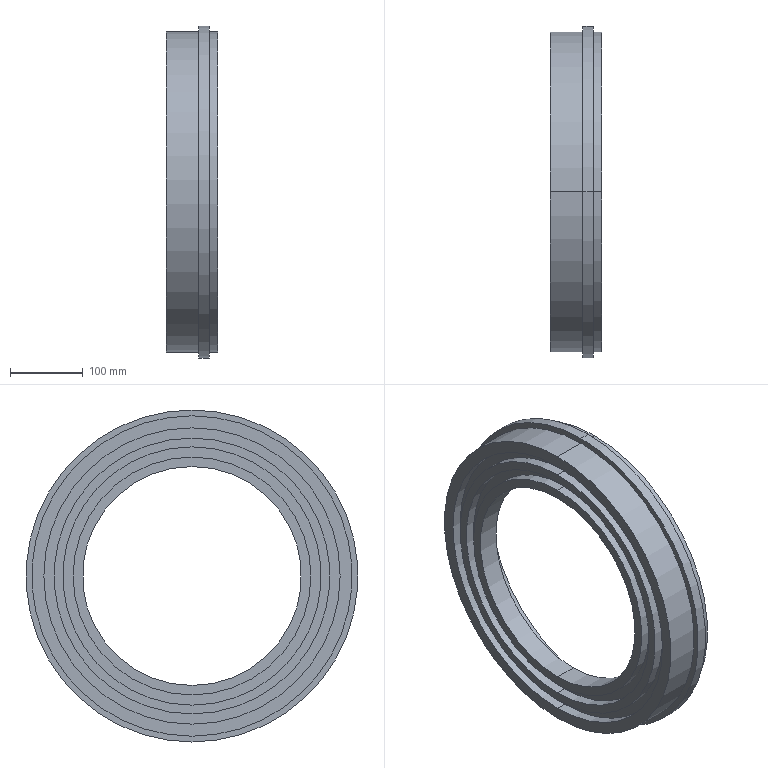Part | SolidWorks | features Revolution 1 | 1 solid | 27 faces | box 71 x 455 x 455 mm | volume 3180516 mm3 | cylinder 18 | plane 9 | commonest cylinder face diameters 439 x4 300 x2 326 x2 354 x2 378 x2 400 x2
STEP:
#1=CARTESIAN_POINT('',(71.,0.,-200.));
#2=VERTEX_POINT('',#1);
#3=CARTESIAN_POINT('',(71.,0.,200.));
#4=VERTEX_POINT('',#3);
#5=CARTESIAN_POINT('',(71.,0.,0.));
#6=DIRECTION('',(-1.,0.,0.));
#7=DIRECTION('',(0.,0.,1.));
#8=AXIS2_PLACEMENT_3D('',#5,#6,#7);
#9=CIRCLE('',#8,200.);
#10=EDGE_CURVE('',#2,#4,#9,.T.);
#11=ORIENTED_EDGE('',*,*,#10,.F.);
#12=CARTESIAN_POINT('',(30.,0.,-200.));
#13=VERTEX_POINT('',#12);
#14=CARTESIAN_POINT('',(0.,0.,-200.));
#15=DIRECTION('',(-1.,0.,0.));
#16=VECTOR('',#15,1000.);
#17=LINE('',#14,#16);
#18=EDGE_CURVE('',#2,#13,#17,.T.);
#19=ORIENTED_EDGE('',*,*,#18,.T.);
#20=CARTESIAN_POINT('',(30.,0.,200.));
#21=VERTEX_POINT('',#20);
#22=CARTESIAN_POINT('',(30.,0.,0.));
#23=DIRECTION('',(-1.,0.,0.));
#24=DIRECTION('',(0.,0.,1.));
#25=AXIS2_PLACEMENT_3D('',#22,#23,#24);
#26=CIRCLE('',#25,200.);
#27=EDGE_CURVE('',#13,#21,#26,.T.);
#28=ORIENTED_EDGE('',*,*,#27,.T.);
#29=CARTESIAN_POINT('',(0.,0.,200.));
#30=DIRECTION('',(-1.,0.,0.));
#31=VECTOR('',#30,1000.);
#32=LINE('',#29,#31);
#33=EDGE_CURVE('',#4,#21,#32,.T.);
#34=ORIENTED_EDGE('',*,*,#33,.F.);
#35=EDGE_LOOP('',(#11,#19,#28,#34));
#36=FACE_OUTER_BOUND('',#35,.T.);
#37=CARTESIAN_POINT('',(0.,0.,0.));
#38=DIRECTION('',(-1.,0.,0.));
#39=DIRECTION('',(0.,0.,1.));
#40=AXIS2_PLACEMENT_3D('',#37,#38,#39);
#41=CYLINDRICAL_SURFACE('',#40,200.);
#42=ADVANCED_FACE('',(#36),#41,.F.);
#43=CARTESIAN_POINT('',(71.,0.,219.5));
#44=VERTEX_POINT('',#43);
#45=CARTESIAN_POINT('',(71.,0.,-219.5));
#46=VERTEX_POINT('',#45);
#47=CARTESIAN_POINT('',(71.,0.,0.));
#48=DIRECTION('',(-1.,0.,0.));
#49=DIRECTION('',(0.,0.,1.));
#50=AXIS2_PLACEMENT_3D('',#47,#48,#49);
#51=CIRCLE('',#50,219.5);
#52=EDGE_CURVE('',#44,#46,#51,.T.);
#53=ORIENTED_EDGE('',*,*,#52,.T.);
#54=CARTESIAN_POINT('',(59.,0.,-219.5));
#55=VERTEX_POINT('',#54);
#56=CARTESIAN_POINT('',(0.,0.,-219.5));
#57=DIRECTION('',(-1.,0.,0.));
#58=VECTOR('',#57,1000.);
#59=LINE('',#56,#58);
#60=EDGE_CURVE('',#46,#55,#59,.T.);
#61=ORIENTED_EDGE('',*,*,#60,.T.);
#62=CARTESIAN_POINT('',(59.,0.,219.5));
#63=VERTEX_POINT('',#62);
#64=CARTESIAN_POINT('',(59.,0.,0.));
#65=DIRECTION('',(-1.,0.,0.));
#66=DIRECTION('',(0.,0.,1.));
#67=AXIS2_PLACEMENT_3D('',#64,#65,#66);
#68=CIRCLE('',#67,219.5);
#69=EDGE_CURVE('',#63,#55,#68,.T.);
#70=ORIENTED_EDGE('',*,*,#69,.F.);
#71=CARTESIAN_POINT('',(0.,0.,219.5));
#72=DIRECTION('',(-1.,0.,0.));
#73=VECTOR('',#72,1000.);
#74=LINE('',#71,#73);
#75=EDGE_CURVE('',#44,#63,#74,.T.);
#76=ORIENTED_EDGE('',*,*,#75,.F.);
#77=EDGE_LOOP('',(#53,#61,#70,#76));
#78=FACE_OUTER_BOUND('',#77,.T.);
#79=CARTESIAN_POINT('',(0.,0.,0.));
#80=DIRECTION('',(-1.,0.,0.));
#81=DIRECTION('',(0.,0.,1.));
#82=AXIS2_PLACEMENT_3D('',#79,#80,#81);
#83=CYLINDRICAL_SURFACE('',#82,219.5);
#84=ADVANCED_FACE('',(#78),#83,.T.);
#85=CARTESIAN_POINT('',(59.,0.,227.5));
#86=VERTEX_POINT('',#85);
#87=CARTESIAN_POINT('',(59.,0.,-227.5));
#88=VERTEX_POINT('',#87);
#89=CARTESIAN_POINT('',(59.,0.,0.));
#90=DIRECTION('',(-1.,0.,0.));
#91=DIRECTION('',(0.,0.,1.));
#92=AXIS2_PLACEMENT_3D('',#89,#90,#91);
#93=CIRCLE('',#92,227.5);
#94=EDGE_CURVE('',#86,#88,#93,.T.);
#95=ORIENTED_EDGE('',*,*,#94,.T.);
#96=CARTESIAN_POINT('',(45.,0.,-227.5));
#97=VERTEX_POINT('',#96);
#98=CARTESIAN_POINT('',(0.,0.,-227.5));
#99=DIRECTION('',(-1.,0.,0.));
#100=VECTOR('',#99,1000.);
#101=LINE('',#98,#100);
#102=EDGE_CURVE('',#88,#97,#101,.T.);
#103=ORIENTED_EDGE('',*,*,#102,.T.);
#104=CARTESIAN_POINT('',(45.,0.,227.5));
#105=VERTEX_POINT('',#104);
#106=CARTESIAN_POINT('',(45.,0.,0.));
#107=DIRECTION('',(-1.,0.,0.));
#108=DIRECTION('',(0.,0.,1.));
#109=AXIS2_PLACEMENT_3D('',#106,#107,#108);
#110=CIRCLE('',#109,227.5);
#111=EDGE_CURVE('',#105,#97,#110,.T.);
#112=ORIENTED_EDGE('',*,*,#111,.F.);
#113=CARTESIAN_POINT('',(0.,0.,227.5));
#114=DIRECTION('',(-1.,0.,0.));
#115=VECTOR('',#114,1000.);
#116=LINE('',#113,#115);
#117=EDGE_CURVE('',#86,#105,#116,.T.);
#118=ORIENTED_EDGE('',*,*,#117,.F.);
#119=EDGE_LOOP('',(#95,#103,#112,#118));
#120=FACE_OUTER_BOUND('',#119,.T.);
#121=CARTESIAN_POINT('',(0.,0.,0.));
#122=DIRECTION('',(-1.,0.,0.));
#123=DIRECTION('',(0.,0.,1.));
#124=AXIS2_PLACEMENT_3D('',#121,#122,#123);
#125=CYLINDRICAL_SURFACE('',#124,227.5);
#126=ADVANCED_FACE('',(#120),#125,.T.);
#127=CARTESIAN_POINT('',(45.,0.,219.5));
#128=VERTEX_POINT('',#127);
#129=CARTESIAN_POINT('',(45.,0.,-219.5));
#130=VERTEX_POINT('',#129);
#131=CARTESIAN_POINT('',(45.,0.,0.));
#132=DIRECTION('',(-1.,0.,0.));
#133=DIRECTION('',(0.,0.,1.));
#134=AXIS2_PLACEMENT_3D('',#131,#132,#133);
#135=CIRCLE('',#134,219.5);
#136=EDGE_CURVE('',#128,#130,#135,.T.);
#137=ORIENTED_EDGE('',*,*,#136,.T.);
#138=CARTESIAN_POINT('',(0.,0.,-219.5));
#139=VERTEX_POINT('',#138);
#140=CARTESIAN_POINT('',(0.,0.,-219.5));
#141=DIRECTION('',(-1.,0.,0.));
#142=VECTOR('',#141,1000.);
#143=LINE('',#140,#142);
#144=EDGE_CURVE('',#130,#139,#143,.T.);
#145=ORIENTED_EDGE('',*,*,#144,.T.);
#146=CARTESIAN_POINT('',(0.,0.,219.5));
#147=VERTEX_POINT('',#146);
#148=CARTESIAN_POINT('',(0.,0.,0.));
#149=DIRECTION('',(-1.,0.,0.));
#150=DIRECTION('',(0.,0.,1.));
#151=AXIS2_PLACEMENT_3D('',#148,#149,#150);
#152=CIRCLE('',#151,219.5);
#153=EDGE_CURVE('',#147,#139,#152,.T.);
#154=ORIENTED_EDGE('',*,*,#153,.F.);
#155=CARTESIAN_POINT('',(0.,0.,219.5));
#156=DIRECTION('',(-1.,0.,0.));
#157=VECTOR('',#156,1000.);
#158=LINE('',#155,#157);
#159=EDGE_CURVE('',#128,#147,#158,.T.);
#160=ORIENTED_EDGE('',*,*,#159,.F.);
#161=EDGE_LOOP('',(#137,#145,#154,#160));
#162=FACE_OUTER_BOUND('',#161,.T.);
#163=CARTESIAN_POINT('',(0.,0.,0.));
#164=DIRECTION('',(-1.,0.,0.));
#165=DIRECTION('',(0.,0.,1.));
#166=AXIS2_PLACEMENT_3D('',#163,#164,#165);
#167=CYLINDRICAL_SURFACE('',#166,219.5);
#168=ADVANCED_FACE('',(#162),#167,.T.);
#169=CARTESIAN_POINT('',(14.,0.,-203.));
#170=VERTEX_POINT('',#169);
#171=CARTESIAN_POINT('',(14.,0.,203.));
#172=VERTEX_POINT('',#171);
#173=CARTESIAN_POINT('',(14.,0.,0.));
#174=DIRECTION('',(-1.,0.,0.));
#175=DIRECTION('',(0.,0.,1.));
#176=AXIS2_PLACEMENT_3D('',#173,#174,#175);
#177=CIRCLE('',#176,203.);
#178=EDGE_CURVE('',#170,#172,#177,.T.);
#179=ORIENTED_EDGE('',*,*,#178,.F.);
#180=CARTESIAN_POINT('',(0.,0.,-203.));
#181=VERTEX_POINT('',#180);
#182=CARTESIAN_POINT('',(0.,0.,-203.));
#183=DIRECTION('',(-1.,0.,0.));
#184=VECTOR('',#183,1000.);
#185=LINE('',#182,#184);
#186=EDGE_CURVE('',#170,#181,#185,.T.);
#187=ORIENTED_EDGE('',*,*,#186,.T.);
#188=CARTESIAN_POINT('',(0.,0.,203.));
#189=VERTEX_POINT('',#188);
#190=CARTESIAN_POINT('',(0.,0.,0.));
#191=DIRECTION('',(-1.,0.,0.));
#192=DIRECTION('',(0.,0.,1.));
#193=AXIS2_PLACEMENT_3D('',#190,#191,#192);
#194=CIRCLE('',#193,203.);
#195=EDGE_CURVE('',#181,#189,#194,.T.);
#196=ORIENTED_EDGE('',*,*,#195,.T.);
#197=CARTESIAN_POINT('',(0.,0.,203.));
#198=DIRECTION('',(-1.,0.,0.));
#199=VECTOR('',#198,1000.);
#200=LINE('',#197,#199);
#201=EDGE_CURVE('',#172,#189,#200,.T.);
#202=ORIENTED_EDGE('',*,*,#201,.F.);
#203=EDGE_LOOP('',(#179,#187,#196,#202));
#204=FACE_OUTER_BOUND('',#203,.T.);
#205=CARTESIAN_POINT('',(0.,0.,0.));
#206=DIRECTION('',(-1.,0.,0.));
#207=DIRECTION('',(0.,0.,1.));
#208=AXIS2_PLACEMENT_3D('',#205,#206,#207);
#209=CYLINDRICAL_SURFACE('',#208,203.);
#210=ADVANCED_FACE('',(#204),#209,.F.);
#211=CARTESIAN_POINT('',(14.,0.,189.));
#212=VERTEX_POINT('',#211);
#213=CARTESIAN_POINT('',(14.,0.,-189.));
#214=VERTEX_POINT('',#213);
#215=CARTESIAN_POINT('',(14.,0.,0.));
#216=DIRECTION('',(-1.,0.,0.));
#217=DIRECTION('',(0.,0.,1.));
#218=AXIS2_PLACEMENT_3D('',#215,#216,#217);
#219=CIRCLE('',#218,189.);
#220=EDGE_CURVE('',#212,#214,#219,.T.);
#221=ORIENTED_EDGE('',*,*,#220,.T.);
#222=CARTESIAN_POINT('',(0.,0.,-189.));
#223=VERTEX_POINT('',#222);
#224=CARTESIAN_POINT('',(0.,0.,-189.));
#225=DIRECTION('',(-1.,0.,0.));
#226=VECTOR('',#225,1000.);
#227=LINE('',#224,#226);
#228=EDGE_CURVE('',#214,#223,#227,.T.);
#229=ORIENTED_EDGE('',*,*,#228,.T.);
#230=CARTESIAN_POINT('',(0.,0.,189.));
#231=VERTEX_POINT('',#230);
#232=CARTESIAN_POINT('',(0.,0.,0.));
#233=DIRECTION('',(-1.,0.,0.));
#234=DIRECTION('',(0.,0.,1.));
#235=AXIS2_PLACEMENT_3D('',#232,#233,#234);
#236=CIRCLE('',#235,189.);
#237=EDGE_CURVE('',#231,#223,#236,.T.);
#238=ORIENTED_EDGE('',*,*,#237,.F.);
#239=CARTESIAN_POINT('',(0.,0.,189.));
#240=DIRECTION('',(-1.,0.,0.));
#241=VECTOR('',#240,1000.);
#242=LINE('',#239,#241);
#243=EDGE_CURVE('',#212,#231,#242,.T.);
#244=ORIENTED_EDGE('',*,*,#243,.F.);
#245=EDGE_LOOP('',(#221,#229,#238,#244));
#246=FACE_OUTER_BOUND('',#245,.T.);
#247=CARTESIAN_POINT('',(0.,0.,0.));
#248=DIRECTION('',(-1.,0.,0.));
#249=DIRECTION('',(0.,0.,1.));
#250=AXIS2_PLACEMENT_3D('',#247,#248,#249);
#251=CYLINDRICAL_SURFACE('',#250,189.);
#252=ADVANCED_FACE('',(#246),#251,.T.);
#253=CARTESIAN_POINT('',(14.,0.,-177.));
#254=VERTEX_POINT('',#253);
#255=CARTESIAN_POINT('',(14.,0.,177.));
#256=VERTEX_POINT('',#255);
#257=CARTESIAN_POINT('',(14.,0.,0.));
#258=DIRECTION('',(-1.,0.,0.));
#259=DIRECTION('',(0.,0.,1.));
#260=AXIS2_PLACEMENT_3D('',#257,#258,#259);
#261=CIRCLE('',#260,177.);
#262=EDGE_CURVE('',#254,#256,#261,.T.);
#263=ORIENTED_EDGE('',*,*,#262,.F.);
#264=CARTESIAN_POINT('',(0.,0.,-177.));
#265=VERTEX_POINT('',#264);
#266=CARTESIAN_POINT('',(0.,0.,-177.));
#267=DIRECTION('',(-1.,0.,0.));
#268=VECTOR('',#267,1000.);
#269=LINE('',#266,#268);
#270=EDGE_CURVE('',#254,#265,#269,.T.);
#271=ORIENTED_EDGE('',*,*,#270,.T.);
#272=CARTESIAN_POINT('',(0.,0.,177.));
#273=VERTEX_POINT('',#272);
#274=CARTESIAN_POINT('',(0.,0.,0.));
#275=DIRECTION('',(-1.,0.,0.));
#276=DIRECTION('',(0.,0.,1.));
#277=AXIS2_PLACEMENT_3D('',#274,#275,#276);
#278=CIRCLE('',#277,177.);
#279=EDGE_CURVE('',#265,#273,#278,.T.);
#280=ORIENTED_EDGE('',*,*,#279,.T.);
#281=CARTESIAN_POINT('',(0.,0.,177.));
#282=DIRECTION('',(-1.,0.,0.));
#283=VECTOR('',#282,1000.);
#284=LINE('',#281,#283);
#285=EDGE_CURVE('',#256,#273,#284,.T.);
#286=ORIENTED_EDGE('',*,*,#285,.F.);
#287=EDGE_LOOP('',(#263,#271,#280,#286));
#288=FACE_OUTER_BOUND('',#287,.T.);
#289=CARTESIAN_POINT('',(0.,0.,0.));
#290=DIRECTION('',(-1.,0.,0.));
#291=DIRECTION('',(0.,0.,1.));
#292=AXIS2_PLACEMENT_3D('',#289,#290,#291);
#293=CYLINDRICAL_SURFACE('',#292,177.);
#294=ADVANCED_FACE('',(#288),#293,.F.);
#295=CARTESIAN_POINT('',(14.,0.,163.));
#296=VERTEX_POINT('',#295);
#297=CARTESIAN_POINT('',(14.,0.,-163.));
#298=VERTEX_POINT('',#297);
#299=CARTESIAN_POINT('',(14.,0.,0.));
#300=DIRECTION('',(-1.,0.,0.));
#301=DIRECTION('',(0.,0.,1.));
#302=AXIS2_PLACEMENT_3D('',#299,#300,#301);
#303=CIRCLE('',#302,163.);
#304=EDGE_CURVE('',#296,#298,#303,.T.);
#305=ORIENTED_EDGE('',*,*,#304,.T.);
#306=CARTESIAN_POINT('',(0.,0.,-163.));
#307=VERTEX_POINT('',#306);
#308=CARTESIAN_POINT('',(0.,0.,-163.));
#309=DIRECTION('',(-1.,0.,0.));
#310=VECTOR('',#309,1000.);
#311=LINE('',#308,#310);
#312=EDGE_CURVE('',#298,#307,#311,.T.);
#313=ORIENTED_EDGE('',*,*,#312,.T.);
#314=CARTESIAN_POINT('',(0.,0.,163.));
#315=VERTEX_POINT('',#314);
#316=CARTESIAN_POINT('',(0.,0.,0.));
#317=DIRECTION('',(-1.,0.,0.));
#318=DIRECTION('',(0.,0.,1.));
#319=AXIS2_PLACEMENT_3D('',#316,#317,#318);
#320=CIRCLE('',#319,163.);
#321=EDGE_CURVE('',#315,#307,#320,.T.);
#322=ORIENTED_EDGE('',*,*,#321,.F.);
#323=CARTESIAN_POINT('',(0.,0.,163.));
#324=DIRECTION('',(-1.,0.,0.));
#325=VECTOR('',#324,1000.);
#326=LINE('',#323,#325);
#327=EDGE_CURVE('',#296,#315,#326,.T.);
#328=ORIENTED_EDGE('',*,*,#327,.F.);
#329=EDGE_LOOP('',(#305,#313,#322,#328));
#330=FACE_OUTER_BOUND('',#329,.T.);
#331=CARTESIAN_POINT('',(0.,0.,0.));
#332=DIRECTION('',(-1.,0.,0.));
#333=DIRECTION('',(0.,0.,1.));
#334=AXIS2_PLACEMENT_3D('',#331,#332,#333);
#335=CYLINDRICAL_SURFACE('',#334,163.);
#336=ADVANCED_FACE('',(#330),#335,.T.);
#337=CARTESIAN_POINT('',(30.,0.,-150.));
#338=VERTEX_POINT('',#337);
#339=CARTESIAN_POINT('',(30.,0.,150.));
#340=VERTEX_POINT('',#339);
#341=CARTESIAN_POINT('',(30.,0.,0.));
#342=DIRECTION('',(-1.,0.,0.));
#343=DIRECTION('',(0.,0.,1.));
#344=AXIS2_PLACEMENT_3D('',#341,#342,#343);
#345=CIRCLE('',#344,150.);
#346=EDGE_CURVE('',#338,#340,#345,.T.);
#347=ORIENTED_EDGE('',*,*,#346,.F.);
#348=CARTESIAN_POINT('',(0.,0.,-150.));
#349=VERTEX_POINT('',#348);
#350=CARTESIAN_POINT('',(0.,0.,-150.));
#351=DIRECTION('',(-1.,0.,0.));
#352=VECTOR('',#351,1000.);
#353=LINE('',#350,#352);
#354=EDGE_CURVE('',#338,#349,#353,.T.);
#355=ORIENTED_EDGE('',*,*,#354,.T.);
#356=CARTESIAN_POINT('',(0.,0.,150.));
#357=VERTEX_POINT('',#356);
#358=CARTESIAN_POINT('',(0.,0.,0.));
#359=DIRECTION('',(-1.,0.,0.));
#360=DIRECTION('',(0.,0.,1.));
#361=AXIS2_PLACEMENT_3D('',#358,#359,#360);
#362=CIRCLE('',#361,150.);
#363=EDGE_CURVE('',#349,#357,#362,.T.);
#364=ORIENTED_EDGE('',*,*,#363,.T.);
#365=CARTESIAN_POINT('',(0.,0.,150.));
#366=DIRECTION('',(-1.,0.,0.));
#367=VECTOR('',#366,1000.);
#368=LINE('',#365,#367);
#369=EDGE_CURVE('',#340,#357,#368,.T.);
#370=ORIENTED_EDGE('',*,*,#369,.F.);
#371=EDGE_LOOP('',(#347,#355,#364,#370));
#372=FACE_OUTER_BOUND('',#371,.T.);
#373=CARTESIAN_POINT('',(0.,0.,0.));
#374=DIRECTION('',(-1.,0.,0.));
#375=DIRECTION('',(0.,0.,1.));
#376=AXIS2_PLACEMENT_3D('',#373,#374,#375);
#377=CYLINDRICAL_SURFACE('',#376,150.);
#378=ADVANCED_FACE('',(#372),#377,.F.);
#379=ORIENTED_EDGE('',*,*,#354,.F.);
#380=CARTESIAN_POINT('',(30.,0.,0.));
#381=DIRECTION('',(-1.,0.,0.));
#382=DIRECTION('',(0.,0.,1.));
#383=AXIS2_PLACEMENT_3D('',#380,#381,#382);
#384=CIRCLE('',#383,150.);
#385=EDGE_CURVE('',#340,#338,#384,.T.);
#386=ORIENTED_EDGE('',*,*,#385,.F.);
#387=ORIENTED_EDGE('',*,*,#369,.T.);
#388=CARTESIAN_POINT('',(0.,0.,0.));
#389=DIRECTION('',(-1.,0.,0.));
#390=DIRECTION('',(0.,0.,1.));
#391=AXIS2_PLACEMENT_3D('',#388,#389,#390);
#392=CIRCLE('',#391,150.);
#393=EDGE_CURVE('',#357,#349,#392,.T.);
#394=ORIENTED_EDGE('',*,*,#393,.T.);
#395=EDGE_LOOP('',(#379,#386,#387,#394));
#396=FACE_OUTER_BOUND('',#395,.T.);
#397=CARTESIAN_POINT('',(0.,0.,0.));
#398=DIRECTION('',(-1.,0.,0.));
#399=DIRECTION('',(0.,0.,1.));
#400=AXIS2_PLACEMENT_3D('',#397,#398,#399);
#401=CYLINDRICAL_SURFACE('',#400,150.);
#402=ADVANCED_FACE('',(#396),#401,.F.);
#403=ORIENTED_EDGE('',*,*,#393,.F.);
#404=ORIENTED_EDGE('',*,*,#363,.F.);
#405=EDGE_LOOP('',(#403,#404));
#406=FACE_BOUND('',#405,.T.);
#407=ORIENTED_EDGE('',*,*,#321,.T.);
#408=CARTESIAN_POINT('',(0.,0.,0.));
#409=DIRECTION('',(-1.,0.,0.));
#410=DIRECTION('',(0.,0.,1.));
#411=AXIS2_PLACEMENT_3D('',#408,#409,#410);
#412=CIRCLE('',#411,163.);
#413=EDGE_CURVE('',#307,#315,#412,.T.);
#414=ORIENTED_EDGE('',*,*,#413,.T.);
#415=EDGE_LOOP('',(#407,#414));
#416=FACE_OUTER_BOUND('',#415,.T.);
#417=CARTESIAN_POINT('',(0.,0.,-150.));
#418=DIRECTION('',(1.,0.,0.));
#419=DIRECTION('',(0.,0.,-1.));
#420=AXIS2_PLACEMENT_3D('',#417,#418,#419);
#421=PLANE('',#420);
#422=ADVANCED_FACE('',(#406,#416),#421,.F.);
#423=ORIENTED_EDGE('',*,*,#312,.F.);
#424=CARTESIAN_POINT('',(14.,0.,0.));
#425=DIRECTION('',(-1.,0.,0.));
#426=DIRECTION('',(0.,0.,1.));
#427=AXIS2_PLACEMENT_3D('',#424,#425,#426);
#428=CIRCLE('',#427,163.);
#429=EDGE_CURVE('',#298,#296,#428,.T.);
#430=ORIENTED_EDGE('',*,*,#429,.T.);
#431=ORIENTED_EDGE('',*,*,#327,.T.);
#432=ORIENTED_EDGE('',*,*,#413,.F.);
#433=EDGE_LOOP('',(#423,#430,#431,#432));
#434=FACE_OUTER_BOUND('',#433,.T.);
#435=CARTESIAN_POINT('',(0.,0.,0.));
#436=DIRECTION('',(-1.,0.,0.));
#437=DIRECTION('',(0.,0.,1.));
#438=AXIS2_PLACEMENT_3D('',#435,#436,#437);
#439=CYLINDRICAL_SURFACE('',#438,163.);
#440=ADVANCED_FACE('',(#434),#439,.T.);
#441=ORIENTED_EDGE('',*,*,#304,.F.);
#442=ORIENTED_EDGE('',*,*,#429,.F.);
#443=EDGE_LOOP('',(#441,#442));
#444=FACE_BOUND('',#443,.T.);
#445=CARTESIAN_POINT('',(14.,0.,0.));
#446=DIRECTION('',(-1.,0.,0.));
#447=DIRECTION('',(0.,0.,1.));
#448=AXIS2_PLACEMENT_3D('',#445,#446,#447);
#449=CIRCLE('',#448,177.);
#450=EDGE_CURVE('',#256,#254,#449,.T.);
#451=ORIENTED_EDGE('',*,*,#450,.T.);
#452=ORIENTED_EDGE('',*,*,#262,.T.);
#453=EDGE_LOOP('',(#451,#452));
#454=FACE_OUTER_BOUND('',#453,.T.);
#455=CARTESIAN_POINT('',(14.,0.,-177.));
#456=DIRECTION('',(1.,0.,0.));
#457=DIRECTION('',(0.,0.,-1.));
#458=AXIS2_PLACEMENT_3D('',#455,#456,#457);
#459=PLANE('',#458);
#460=ADVANCED_FACE('',(#444,#454),#459,.F.);
#461=ORIENTED_EDGE('',*,*,#270,.F.);
#462=ORIENTED_EDGE('',*,*,#450,.F.);
#463=ORIENTED_EDGE('',*,*,#285,.T.);
#464=CARTESIAN_POINT('',(0.,0.,0.));
#465=DIRECTION('',(-1.,0.,0.));
#466=DIRECTION('',(0.,0.,1.));
#467=AXIS2_PLACEMENT_3D('',#464,#465,#466);
#468=CIRCLE('',#467,177.);
#469=EDGE_CURVE('',#273,#265,#468,.T.);
#470=ORIENTED_EDGE('',*,*,#469,.T.);
#471=EDGE_LOOP('',(#461,#462,#463,#470));
#472=FACE_OUTER_BOUND('',#471,.T.);
#473=CARTESIAN_POINT('',(0.,0.,0.));
#474=DIRECTION('',(-1.,0.,0.));
#475=DIRECTION('',(0.,0.,1.));
#476=AXIS2_PLACEMENT_3D('',#473,#474,#475);
#477=CYLINDRICAL_SURFACE('',#476,177.);
#478=ADVANCED_FACE('',(#472),#477,.F.);
#479=ORIENTED_EDGE('',*,*,#469,.F.);
#480=ORIENTED_EDGE('',*,*,#279,.F.);
#481=EDGE_LOOP('',(#479,#480));
#482=FACE_BOUND('',#481,.T.);
#483=ORIENTED_EDGE('',*,*,#237,.T.);
#484=CARTESIAN_POINT('',(0.,0.,0.));
#485=DIRECTION('',(-1.,0.,0.));
#486=DIRECTION('',(0.,0.,1.));
#487=AXIS2_PLACEMENT_3D('',#484,#485,#486);
#488=CIRCLE('',#487,189.);
#489=EDGE_CURVE('',#223,#231,#488,.T.);
#490=ORIENTED_EDGE('',*,*,#489,.T.);
#491=EDGE_LOOP('',(#483,#490));
#492=FACE_OUTER_BOUND('',#491,.T.);
#493=CARTESIAN_POINT('',(0.,0.,-177.));
#494=DIRECTION('',(1.,0.,0.));
#495=DIRECTION('',(0.,0.,-1.));
#496=AXIS2_PLACEMENT_3D('',#493,#494,#495);
#497=PLANE('',#496);
#498=ADVANCED_FACE('',(#482,#492),#497,.F.);
#499=ORIENTED_EDGE('',*,*,#228,.F.);
#500=CARTESIAN_POINT('',(14.,0.,0.));
#501=DIRECTION('',(-1.,0.,0.));
#502=DIRECTION('',(0.,0.,1.));
#503=AXIS2_PLACEMENT_3D('',#500,#501,#502);
#504=CIRCLE('',#503,189.);
#505=EDGE_CURVE('',#214,#212,#504,.T.);
#506=ORIENTED_EDGE('',*,*,#505,.T.);
#507=ORIENTED_EDGE('',*,*,#243,.T.);
#508=ORIENTED_EDGE('',*,*,#489,.F.);
#509=EDGE_LOOP('',(#499,#506,#507,#508));
#510=FACE_OUTER_BOUND('',#509,.T.);
#511=CARTESIAN_POINT('',(0.,0.,0.));
#512=DIRECTION('',(-1.,0.,0.));
#513=DIRECTION('',(0.,0.,1.));
#514=AXIS2_PLACEMENT_3D('',#511,#512,#513);
#515=CYLINDRICAL_SURFACE('',#514,189.);
#516=ADVANCED_FACE('',(#510),#515,.T.);
#517=ORIENTED_EDGE('',*,*,#220,.F.);
#518=ORIENTED_EDGE('',*,*,#505,.F.);
#519=EDGE_LOOP('',(#517,#518));
#520=FACE_BOUND('',#519,.T.);
#521=CARTESIAN_POINT('',(14.,0.,0.));
#522=DIRECTION('',(-1.,0.,0.));
#523=DIRECTION('',(0.,0.,1.));
#524=AXIS2_PLACEMENT_3D('',#521,#522,#523);
#525=CIRCLE('',#524,203.);
#526=EDGE_CURVE('',#172,#170,#525,.T.);
#527=ORIENTED_EDGE('',*,*,#526,.T.);
#528=ORIENTED_EDGE('',*,*,#178,.T.);
#529=EDGE_LOOP('',(#527,#528));
#530=FACE_OUTER_BOUND('',#529,.T.);
#531=CARTESIAN_POINT('',(14.,0.,-203.));
#532=DIRECTION('',(1.,0.,0.));
#533=DIRECTION('',(0.,0.,-1.));
#534=AXIS2_PLACEMENT_3D('',#531,#532,#533);
#535=PLANE('',#534);
#536=ADVANCED_FACE('',(#520,#530),#535,.F.);
#537=ORIENTED_EDGE('',*,*,#186,.F.);
#538=ORIENTED_EDGE('',*,*,#526,.F.);
#539=ORIENTED_EDGE('',*,*,#201,.T.);
#540=CARTESIAN_POINT('',(0.,0.,0.));
#541=DIRECTION('',(-1.,0.,0.));
#542=DIRECTION('',(0.,0.,1.));
#543=AXIS2_PLACEMENT_3D('',#540,#541,#542);
#544=CIRCLE('',#543,203.);
#545=EDGE_CURVE('',#189,#181,#544,.T.);
#546=ORIENTED_EDGE('',*,*,#545,.T.);
#547=EDGE_LOOP('',(#537,#538,#539,#546));
#548=FACE_OUTER_BOUND('',#547,.T.);
#549=CARTESIAN_POINT('',(0.,0.,0.));
#550=DIRECTION('',(-1.,0.,0.));
#551=DIRECTION('',(0.,0.,1.));
#552=AXIS2_PLACEMENT_3D('',#549,#550,#551);
#553=CYLINDRICAL_SURFACE('',#552,203.);
#554=ADVANCED_FACE('',(#548),#553,.F.);
#555=ORIENTED_EDGE('',*,*,#545,.F.);
#556=ORIENTED_EDGE('',*,*,#195,.F.);
#557=EDGE_LOOP('',(#555,#556));
#558=FACE_BOUND('',#557,.T.);
#559=ORIENTED_EDGE('',*,*,#153,.T.);
#560=CARTESIAN_POINT('',(0.,0.,0.));
#561=DIRECTION('',(-1.,0.,0.));
#562=DIRECTION('',(0.,0.,1.));
#563=AXIS2_PLACEMENT_3D('',#560,#561,#562);
#564=CIRCLE('',#563,219.5);
#565=EDGE_CURVE('',#139,#147,#564,.T.);
#566=ORIENTED_EDGE('',*,*,#565,.T.);
#567=EDGE_LOOP('',(#559,#566));
#568=FACE_OUTER_BOUND('',#567,.T.);
#569=CARTESIAN_POINT('',(0.,0.,-203.));
#570=DIRECTION('',(1.,0.,0.));
#571=DIRECTION('',(0.,0.,-1.));
#572=AXIS2_PLACEMENT_3D('',#569,#570,#571);
#573=PLANE('',#572);
#574=ADVANCED_FACE('',(#558,#568),#573,.F.);
#575=ORIENTED_EDGE('',*,*,#144,.F.);
#576=CARTESIAN_POINT('',(45.,0.,0.));
#577=DIRECTION('',(-1.,0.,0.));
#578=DIRECTION('',(0.,0.,1.));
#579=AXIS2_PLACEMENT_3D('',#576,#577,#578);
#580=CIRCLE('',#579,219.5);
#581=EDGE_CURVE('',#130,#128,#580,.T.);
#582=ORIENTED_EDGE('',*,*,#581,.T.);
#583=ORIENTED_EDGE('',*,*,#159,.T.);
#584=ORIENTED_EDGE('',*,*,#565,.F.);
#585=EDGE_LOOP('',(#575,#582,#583,#584));
#586=FACE_OUTER_BOUND('',#585,.T.);
#587=CARTESIAN_POINT('',(0.,0.,0.));
#588=DIRECTION('',(-1.,0.,0.));
#589=DIRECTION('',(0.,0.,1.));
#590=AXIS2_PLACEMENT_3D('',#587,#588,#589);
#591=CYLINDRICAL_SURFACE('',#590,219.5);
#592=ADVANCED_FACE('',(#586),#591,.T.);
#593=ORIENTED_EDGE('',*,*,#136,.F.);
#594=ORIENTED_EDGE('',*,*,#581,.F.);
#595=EDGE_LOOP('',(#593,#594));
#596=FACE_BOUND('',#595,.T.);
#597=ORIENTED_EDGE('',*,*,#111,.T.);
#598=CARTESIAN_POINT('',(45.,0.,0.));
#599=DIRECTION('',(-1.,0.,0.));
#600=DIRECTION('',(0.,0.,1.));
#601=AXIS2_PLACEMENT_3D('',#598,#599,#600);
#602=CIRCLE('',#601,227.5);
#603=EDGE_CURVE('',#97,#105,#602,.T.);
#604=ORIENTED_EDGE('',*,*,#603,.T.);
#605=EDGE_LOOP('',(#597,#604));
#606=FACE_OUTER_BOUND('',#605,.T.);
#607=CARTESIAN_POINT('',(45.,0.,-219.5));
#608=DIRECTION('',(1.,0.,0.));
#609=DIRECTION('',(0.,0.,-1.));
#610=AXIS2_PLACEMENT_3D('',#607,#608,#609);
#611=PLANE('',#610);
#612=ADVANCED_FACE('',(#596,#606),#611,.F.);
#613=ORIENTED_EDGE('',*,*,#102,.F.);
#614=CARTESIAN_POINT('',(59.,0.,0.));
#615=DIRECTION('',(-1.,0.,0.));
#616=DIRECTION('',(0.,0.,1.));
#617=AXIS2_PLACEMENT_3D('',#614,#615,#616);
#618=CIRCLE('',#617,227.5);
#619=EDGE_CURVE('',#88,#86,#618,.T.);
#620=ORIENTED_EDGE('',*,*,#619,.T.);
#621=ORIENTED_EDGE('',*,*,#117,.T.);
#622=ORIENTED_EDGE('',*,*,#603,.F.);
#623=EDGE_LOOP('',(#613,#620,#621,#622));
#624=FACE_OUTER_BOUND('',#623,.T.);
#625=CARTESIAN_POINT('',(0.,0.,0.));
#626=DIRECTION('',(-1.,0.,0.));
#627=DIRECTION('',(0.,0.,1.));
#628=AXIS2_PLACEMENT_3D('',#625,#626,#627);
#629=CYLINDRICAL_SURFACE('',#628,227.5);
#630=ADVANCED_FACE('',(#624),#629,.T.);
#631=ORIENTED_EDGE('',*,*,#94,.F.);
#632=ORIENTED_EDGE('',*,*,#619,.F.);
#633=EDGE_LOOP('',(#631,#632));
#634=FACE_OUTER_BOUND('',#633,.T.);
#635=ORIENTED_EDGE('',*,*,#69,.T.);
#636=CARTESIAN_POINT('',(59.,0.,0.));
#637=DIRECTION('',(-1.,0.,0.));
#638=DIRECTION('',(0.,0.,1.));
#639=AXIS2_PLACEMENT_3D('',#636,#637,#638);
#640=CIRCLE('',#639,219.5);
#641=EDGE_CURVE('',#55,#63,#640,.T.);
#642=ORIENTED_EDGE('',*,*,#641,.T.);
#643=EDGE_LOOP('',(#635,#642));
#644=FACE_BOUND('',#643,.T.);
#645=CARTESIAN_POINT('',(59.,0.,-227.5));
#646=DIRECTION('',(-1.,0.,0.));
#647=DIRECTION('',(0.,0.,1.));
#648=AXIS2_PLACEMENT_3D('',#645,#646,#647);
#649=PLANE('',#648);
#650=ADVANCED_FACE('',(#634,#644),#649,.F.);
#651=ORIENTED_EDGE('',*,*,#60,.F.);
#652=CARTESIAN_POINT('',(71.,0.,0.));
#653=DIRECTION('',(-1.,0.,0.));
#654=DIRECTION('',(0.,0.,1.));
#655=AXIS2_PLACEMENT_3D('',#652,#653,#654);
#656=CIRCLE('',#655,219.5);
#657=EDGE_CURVE('',#46,#44,#656,.T.);
#658=ORIENTED_EDGE('',*,*,#657,.T.);
#659=ORIENTED_EDGE('',*,*,#75,.T.);
#660=ORIENTED_EDGE('',*,*,#641,.F.);
#661=EDGE_LOOP('',(#651,#658,#659,#660));
#662=FACE_OUTER_BOUND('',#661,.T.);
#663=CARTESIAN_POINT('',(0.,0.,0.));
#664=DIRECTION('',(-1.,0.,0.));
#665=DIRECTION('',(0.,0.,1.));
#666=AXIS2_PLACEMENT_3D('',#663,#664,#665);
#667=CYLINDRICAL_SURFACE('',#666,219.5);
#668=ADVANCED_FACE('',(#662),#667,.T.);
#669=ORIENTED_EDGE('',*,*,#52,.F.);
#670=ORIENTED_EDGE('',*,*,#657,.F.);
#671=EDGE_LOOP('',(#669,#670));
#672=FACE_OUTER_BOUND('',#671,.T.);
#673=CARTESIAN_POINT('',(71.,0.,0.));
#674=DIRECTION('',(-1.,0.,0.));
#675=DIRECTION('',(0.,0.,1.));
#676=AXIS2_PLACEMENT_3D('',#673,#674,#675);
#677=CIRCLE('',#676,200.);
#678=EDGE_CURVE('',#4,#2,#677,.T.);
#679=ORIENTED_EDGE('',*,*,#678,.T.);
#680=ORIENTED_EDGE('',*,*,#10,.T.);
#681=EDGE_LOOP('',(#679,#680));
#682=FACE_BOUND('',#681,.T.);
#683=CARTESIAN_POINT('',(71.,0.,-219.5));
#684=DIRECTION('',(-1.,0.,0.));
#685=DIRECTION('',(0.,0.,1.));
#686=AXIS2_PLACEMENT_3D('',#683,#684,#685);
#687=PLANE('',#686);
#688=ADVANCED_FACE('',(#672,#682),#687,.F.);
#689=ORIENTED_EDGE('',*,*,#18,.F.);
#690=ORIENTED_EDGE('',*,*,#678,.F.);
#691=ORIENTED_EDGE('',*,*,#33,.T.);
#692=CARTESIAN_POINT('',(30.,0.,0.));
#693=DIRECTION('',(-1.,0.,0.));
#694=DIRECTION('',(0.,0.,1.));
#695=AXIS2_PLACEMENT_3D('',#692,#693,#694);
#696=CIRCLE('',#695,200.);
#697=EDGE_CURVE('',#21,#13,#696,.T.);
#698=ORIENTED_EDGE('',*,*,#697,.T.);
#699=EDGE_LOOP('',(#689,#690,#691,#698));
#700=FACE_OUTER_BOUND('',#699,.T.);
#701=CARTESIAN_POINT('',(0.,0.,0.));
#702=DIRECTION('',(-1.,0.,0.));
#703=DIRECTION('',(0.,0.,1.));
#704=AXIS2_PLACEMENT_3D('',#701,#702,#703);
#705=CYLINDRICAL_SURFACE('',#704,200.);
#706=ADVANCED_FACE('',(#700),#705,.F.);
#707=ORIENTED_EDGE('',*,*,#697,.F.);
#708=ORIENTED_EDGE('',*,*,#27,.F.);
#709=EDGE_LOOP('',(#707,#708));
#710=FACE_OUTER_BOUND('',#709,.T.);
#711=ORIENTED_EDGE('',*,*,#385,.T.);
#712=ORIENTED_EDGE('',*,*,#346,.T.);
#713=EDGE_LOOP('',(#711,#712));
#714=FACE_BOUND('',#713,.T.);
#715=CARTESIAN_POINT('',(30.,0.,-200.));
#716=DIRECTION('',(-1.,0.,0.));
#717=DIRECTION('',(0.,0.,1.));
#718=AXIS2_PLACEMENT_3D('',#715,#716,#717);
#719=PLANE('',#718);
#720=ADVANCED_FACE('',(#710,#714),#719,.F.);
#721=CLOSED_SHELL('',(#42,#84,#126,#168,#210,#252,#294,#336,#378,#402,#422,#440,#460,#478,#498,#516,#536,#554,#574,#592,#612,#630,#650,#668,#688,#706,#720));
#722=MANIFOLD_SOLID_BREP('',#721);
#723=CARTESIAN_POINT('',(0.,0.,0.));
#724=DIRECTION('',(0.,0.,1.));
#725=DIRECTION('',(1.,0.,0.));
#726=AXIS2_PLACEMENT_3D('',#723,#724,#725);
#727=(LENGTH_UNIT()NAMED_UNIT(*)SI_UNIT(.MILLI.,.METRE.));
#728=UNCERTAINTY_MEASURE_WITH_UNIT(LENGTH_MEASURE(0.00001),#727,'','');
#729=(NAMED_UNIT(*)PLANE_ANGLE_UNIT()SI_UNIT($,.RADIAN.));
#730=(NAMED_UNIT(*)SI_UNIT($,.STERADIAN.)SOLID_ANGLE_UNIT());
#731=(GEOMETRIC_REPRESENTATION_CONTEXT(3)GLOBAL_UNCERTAINTY_ASSIGNED_CONTEXT((#728))GLOBAL_UNIT_ASSIGNED_CONTEXT((#727,#729,#730))REPRESENTATION_CONTEXT('',''));
#732=ADVANCED_BREP_SHAPE_REPRESENTATION('',(#722,#726),#731);